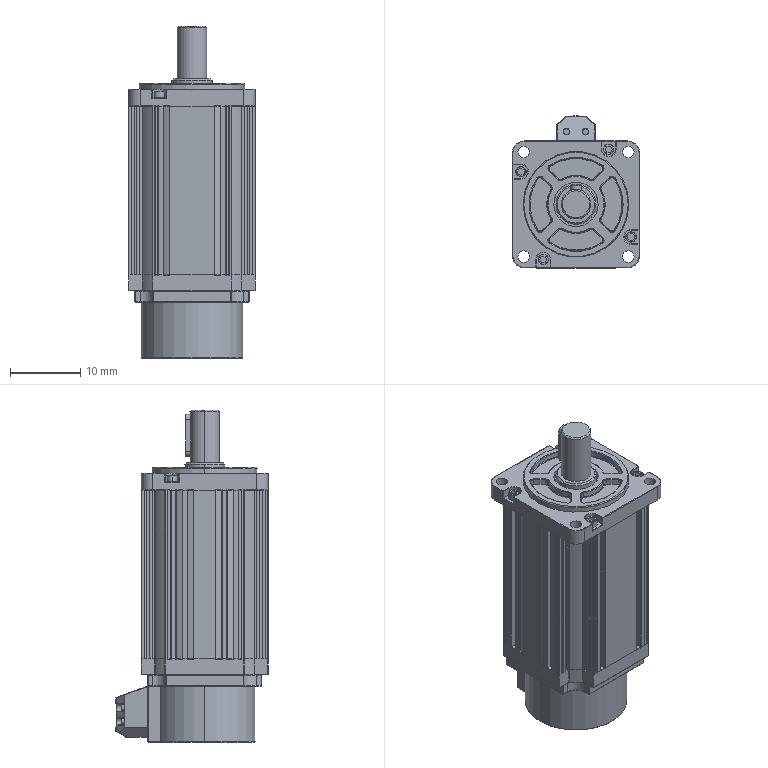Part | SolidWorks | features BaseBody 1, Scale 1 | 1 solid | 975 faces | box 18 x 21.6 x 47.1 mm | volume 10038 mm3 | plane 393 | cylinder 362 | torus 137 | sphere 52 | spline 24 | cone 7 | commonest cylinder face diameters 0.12 x216 0.9 x20 18 x20 0.18 x16 0.762 x8 1.08 x8